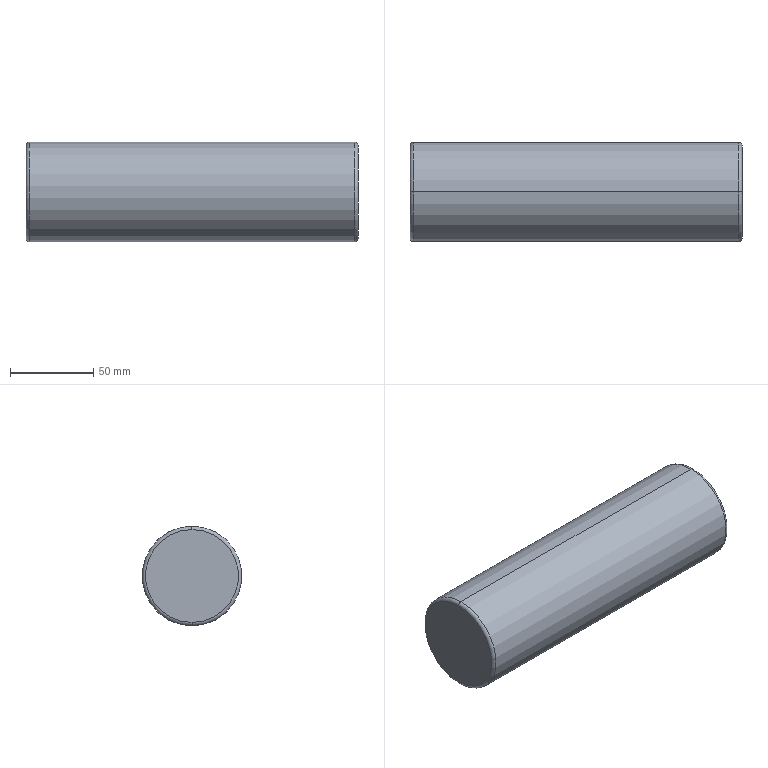Part | SolidWorks | features Extrusion 1, Fillet 1 | 1 solid | 8 faces | box 200 x 60 x 60 mm | volume 565168 mm3 | torus 4 | cylinder 2 | plane 2 | commonest cylinder face diameters 60 x2
STEP:
#1=CARTESIAN_POINT('',(198.,0.,30.));
#2=VERTEX_POINT('',#1);
#3=CARTESIAN_POINT('',(198.,0.,-30.));
#4=VERTEX_POINT('',#3);
#5=CARTESIAN_POINT('',(198.,0.,0.));
#6=DIRECTION('',(-1.,0.,0.));
#7=DIRECTION('',(0.,0.,-1.));
#8=AXIS2_PLACEMENT_3D('',#5,#6,#7);
#9=CIRCLE('',#8,30.);
#10=EDGE_CURVE('',#2,#4,#9,.T.);
#11=ORIENTED_EDGE('',*,*,#10,.F.);
#12=CARTESIAN_POINT('',(200.,0.,28.));
#13=VERTEX_POINT('',#12);
#14=CARTESIAN_POINT('',(198.,0.,28.));
#15=DIRECTION('',(0.,1.,0.));
#16=DIRECTION('',(0.,0.,1.));
#17=AXIS2_PLACEMENT_3D('',#14,#15,#16);
#18=CIRCLE('',#17,2.);
#19=EDGE_CURVE('',#2,#13,#18,.T.);
#20=ORIENTED_EDGE('',*,*,#19,.T.);
#21=CARTESIAN_POINT('',(200.,0.,-28.));
#22=VERTEX_POINT('',#21);
#23=CARTESIAN_POINT('',(200.,0.,0.));
#24=DIRECTION('',(1.,0.,0.));
#25=DIRECTION('',(0.,0.,-1.));
#26=AXIS2_PLACEMENT_3D('',#23,#24,#25);
#27=CIRCLE('',#26,28.);
#28=EDGE_CURVE('',#22,#13,#27,.T.);
#29=ORIENTED_EDGE('',*,*,#28,.F.);
#30=CARTESIAN_POINT('',(198.,0.,-28.));
#31=DIRECTION('',(0.,-1.,0.));
#32=DIRECTION('',(0.,0.,-1.));
#33=AXIS2_PLACEMENT_3D('',#30,#31,#32);
#34=CIRCLE('',#33,2.);
#35=EDGE_CURVE('',#4,#22,#34,.T.);
#36=ORIENTED_EDGE('',*,*,#35,.F.);
#37=EDGE_LOOP('',(#11,#20,#29,#36));
#38=FACE_OUTER_BOUND('',#37,.T.);
#39=CARTESIAN_POINT('',(198.,0.,0.));
#40=DIRECTION('',(1.,0.,0.));
#41=DIRECTION('',(0.,0.,-1.));
#42=AXIS2_PLACEMENT_3D('',#39,#40,#41);
#43=TOROIDAL_SURFACE('',#42,28.,2.);
#44=ADVANCED_FACE('',(#38),#43,.T.);
#45=CARTESIAN_POINT('',(0.,0.,28.));
#46=VERTEX_POINT('',#45);
#47=CARTESIAN_POINT('',(0.,0.,-28.));
#48=VERTEX_POINT('',#47);
#49=CARTESIAN_POINT('',(0.,0.,0.));
#50=DIRECTION('',(-1.,0.,0.));
#51=DIRECTION('',(0.,0.,-1.));
#52=AXIS2_PLACEMENT_3D('',#49,#50,#51);
#53=CIRCLE('',#52,28.);
#54=EDGE_CURVE('',#46,#48,#53,.T.);
#55=ORIENTED_EDGE('',*,*,#54,.F.);
#56=CARTESIAN_POINT('',(2.,0.,30.));
#57=VERTEX_POINT('',#56);
#58=CARTESIAN_POINT('',(2.,0.,28.));
#59=DIRECTION('',(0.,1.,0.));
#60=DIRECTION('',(0.,0.,1.));
#61=AXIS2_PLACEMENT_3D('',#58,#59,#60);
#62=CIRCLE('',#61,2.);
#63=EDGE_CURVE('',#46,#57,#62,.T.);
#64=ORIENTED_EDGE('',*,*,#63,.T.);
#65=CARTESIAN_POINT('',(2.,0.,-30.));
#66=VERTEX_POINT('',#65);
#67=CARTESIAN_POINT('',(2.,0.,0.));
#68=DIRECTION('',(1.,0.,0.));
#69=DIRECTION('',(0.,0.,-1.));
#70=AXIS2_PLACEMENT_3D('',#67,#68,#69);
#71=CIRCLE('',#70,30.);
#72=EDGE_CURVE('',#66,#57,#71,.T.);
#73=ORIENTED_EDGE('',*,*,#72,.F.);
#74=CARTESIAN_POINT('',(2.,0.,-28.));
#75=DIRECTION('',(0.,-1.,0.));
#76=DIRECTION('',(0.,0.,-1.));
#77=AXIS2_PLACEMENT_3D('',#74,#75,#76);
#78=CIRCLE('',#77,2.);
#79=EDGE_CURVE('',#48,#66,#78,.T.);
#80=ORIENTED_EDGE('',*,*,#79,.F.);
#81=EDGE_LOOP('',(#55,#64,#73,#80));
#82=FACE_OUTER_BOUND('',#81,.T.);
#83=CARTESIAN_POINT('',(2.,0.,0.));
#84=DIRECTION('',(1.,0.,0.));
#85=DIRECTION('',(0.,0.,-1.));
#86=AXIS2_PLACEMENT_3D('',#83,#84,#85);
#87=TOROIDAL_SURFACE('',#86,28.,2.);
#88=ADVANCED_FACE('',(#82),#87,.T.);
#89=ORIENTED_EDGE('',*,*,#10,.T.);
#90=CARTESIAN_POINT('',(200.,0.,-30.));
#91=DIRECTION('',(-1.,0.,0.));
#92=VECTOR('',#91,1000.);
#93=LINE('',#90,#92);
#94=EDGE_CURVE('',#4,#66,#93,.T.);
#95=ORIENTED_EDGE('',*,*,#94,.T.);
#96=ORIENTED_EDGE('',*,*,#72,.T.);
#97=CARTESIAN_POINT('',(200.,0.,30.));
#98=DIRECTION('',(-1.,0.,0.));
#99=VECTOR('',#98,1000.);
#100=LINE('',#97,#99);
#101=EDGE_CURVE('',#2,#57,#100,.T.);
#102=ORIENTED_EDGE('',*,*,#101,.F.);
#103=EDGE_LOOP('',(#89,#95,#96,#102));
#104=FACE_OUTER_BOUND('',#103,.T.);
#105=CARTESIAN_POINT('',(200.,0.,0.));
#106=DIRECTION('',(-1.,0.,0.));
#107=DIRECTION('',(0.,0.,1.));
#108=AXIS2_PLACEMENT_3D('',#105,#106,#107);
#109=CYLINDRICAL_SURFACE('',#108,30.);
#110=ADVANCED_FACE('',(#104),#109,.T.);
#111=ORIENTED_EDGE('',*,*,#94,.F.);
#112=CARTESIAN_POINT('',(198.,0.,0.));
#113=DIRECTION('',(-1.,0.,0.));
#114=DIRECTION('',(0.,0.,-1.));
#115=AXIS2_PLACEMENT_3D('',#112,#113,#114);
#116=CIRCLE('',#115,30.);
#117=EDGE_CURVE('',#4,#2,#116,.T.);
#118=ORIENTED_EDGE('',*,*,#117,.T.);
#119=ORIENTED_EDGE('',*,*,#101,.T.);
#120=CARTESIAN_POINT('',(2.,0.,0.));
#121=DIRECTION('',(1.,0.,0.));
#122=DIRECTION('',(0.,0.,-1.));
#123=AXIS2_PLACEMENT_3D('',#120,#121,#122);
#124=CIRCLE('',#123,30.);
#125=EDGE_CURVE('',#57,#66,#124,.T.);
#126=ORIENTED_EDGE('',*,*,#125,.T.);
#127=EDGE_LOOP('',(#111,#118,#119,#126));
#128=FACE_OUTER_BOUND('',#127,.T.);
#129=CARTESIAN_POINT('',(200.,0.,0.));
#130=DIRECTION('',(-1.,0.,0.));
#131=DIRECTION('',(0.,0.,1.));
#132=AXIS2_PLACEMENT_3D('',#129,#130,#131);
#133=CYLINDRICAL_SURFACE('',#132,30.);
#134=ADVANCED_FACE('',(#128),#133,.T.);
#135=ORIENTED_EDGE('',*,*,#28,.T.);
#136=CARTESIAN_POINT('',(200.,0.,0.));
#137=DIRECTION('',(1.,0.,0.));
#138=DIRECTION('',(0.,0.,-1.));
#139=AXIS2_PLACEMENT_3D('',#136,#137,#138);
#140=CIRCLE('',#139,28.);
#141=EDGE_CURVE('',#13,#22,#140,.T.);
#142=ORIENTED_EDGE('',*,*,#141,.T.);
#143=EDGE_LOOP('',(#135,#142));
#144=FACE_OUTER_BOUND('',#143,.T.);
#145=CARTESIAN_POINT('',(200.,0.,0.));
#146=DIRECTION('',(1.,0.,0.));
#147=DIRECTION('',(0.,0.,-1.));
#148=AXIS2_PLACEMENT_3D('',#145,#146,#147);
#149=PLANE('',#148);
#150=ADVANCED_FACE('',(#144),#149,.T.);
#151=CARTESIAN_POINT('',(0.,0.,0.));
#152=DIRECTION('',(-1.,0.,0.));
#153=DIRECTION('',(0.,0.,-1.));
#154=AXIS2_PLACEMENT_3D('',#151,#152,#153);
#155=CIRCLE('',#154,28.);
#156=EDGE_CURVE('',#48,#46,#155,.T.);
#157=ORIENTED_EDGE('',*,*,#156,.T.);
#158=ORIENTED_EDGE('',*,*,#54,.T.);
#159=EDGE_LOOP('',(#157,#158));
#160=FACE_OUTER_BOUND('',#159,.T.);
#161=CARTESIAN_POINT('',(0.,0.,0.));
#162=DIRECTION('',(1.,0.,0.));
#163=DIRECTION('',(0.,0.,-1.));
#164=AXIS2_PLACEMENT_3D('',#161,#162,#163);
#165=PLANE('',#164);
#166=ADVANCED_FACE('',(#160),#165,.F.);
#167=ORIENTED_EDGE('',*,*,#63,.F.);
#168=ORIENTED_EDGE('',*,*,#156,.F.);
#169=ORIENTED_EDGE('',*,*,#79,.T.);
#170=ORIENTED_EDGE('',*,*,#125,.F.);
#171=EDGE_LOOP('',(#167,#168,#169,#170));
#172=FACE_OUTER_BOUND('',#171,.T.);
#173=CARTESIAN_POINT('',(2.,0.,0.));
#174=DIRECTION('',(1.,0.,0.));
#175=DIRECTION('',(0.,0.,-1.));
#176=AXIS2_PLACEMENT_3D('',#173,#174,#175);
#177=TOROIDAL_SURFACE('',#176,28.,2.);
#178=ADVANCED_FACE('',(#172),#177,.T.);
#179=ORIENTED_EDGE('',*,*,#19,.F.);
#180=ORIENTED_EDGE('',*,*,#117,.F.);
#181=ORIENTED_EDGE('',*,*,#35,.T.);
#182=ORIENTED_EDGE('',*,*,#141,.F.);
#183=EDGE_LOOP('',(#179,#180,#181,#182));
#184=FACE_OUTER_BOUND('',#183,.T.);
#185=CARTESIAN_POINT('',(198.,0.,0.));
#186=DIRECTION('',(1.,0.,0.));
#187=DIRECTION('',(0.,0.,-1.));
#188=AXIS2_PLACEMENT_3D('',#185,#186,#187);
#189=TOROIDAL_SURFACE('',#188,28.,2.);
#190=ADVANCED_FACE('',(#184),#189,.T.);
#191=CLOSED_SHELL('',(#44,#88,#110,#134,#150,#166,#178,#190));
#192=MANIFOLD_SOLID_BREP('',#191);
#193=CARTESIAN_POINT('',(0.,0.,0.));
#194=DIRECTION('',(0.,0.,1.));
#195=DIRECTION('',(1.,0.,0.));
#196=AXIS2_PLACEMENT_3D('',#193,#194,#195);
#197=(LENGTH_UNIT()NAMED_UNIT(*)SI_UNIT(.MILLI.,.METRE.));
#198=UNCERTAINTY_MEASURE_WITH_UNIT(LENGTH_MEASURE(0.00001),#197,'','');
#199=(NAMED_UNIT(*)PLANE_ANGLE_UNIT()SI_UNIT($,.RADIAN.));
#200=(NAMED_UNIT(*)SI_UNIT($,.STERADIAN.)SOLID_ANGLE_UNIT());
#201=(GEOMETRIC_REPRESENTATION_CONTEXT(3)GLOBAL_UNCERTAINTY_ASSIGNED_CONTEXT((#198))GLOBAL_UNIT_ASSIGNED_CONTEXT((#197,#199,#200))REPRESENTATION_CONTEXT('',''));
#202=ADVANCED_BREP_SHAPE_REPRESENTATION('',(#192,#196),#201);